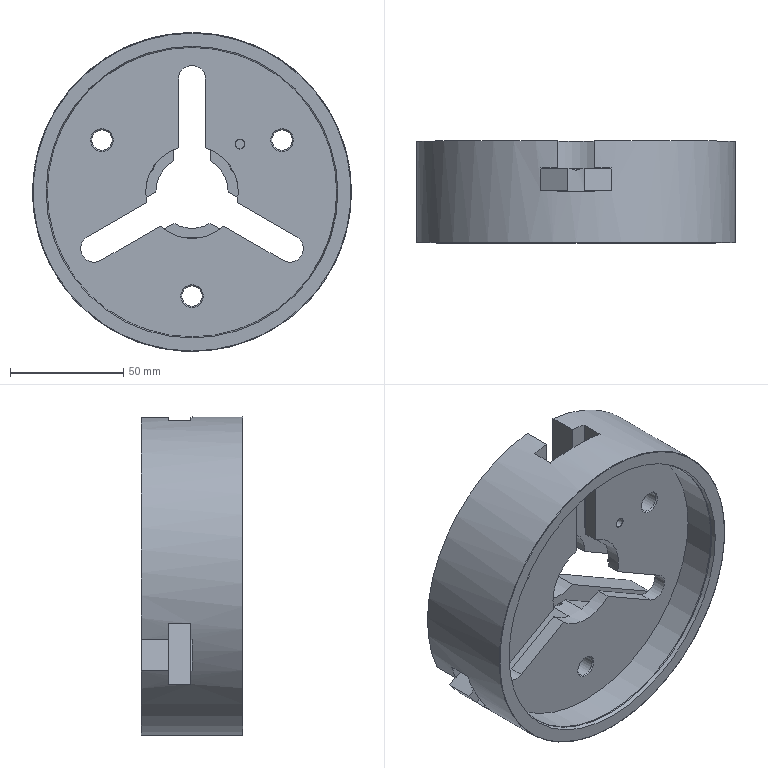NC program | NX | posted with a generic post | part box 141 x 45 x 141 mm
Whole program:
N10 G17 G21 G94 G90
(PLANAR_MILL_2_COPY , TOOL : D30)
N12 T07 M6
N14 G54
N16 G17 G0 G90 X0. Y110. S0 M3
N18 G43 Z100. H7
N20 Z-20.1
N22 G94 G1 Z-21.1 F250.
N24 Y80.
N26 X0.4
N28 Y15.1
N30 X-0.4
N32 Y80.
N34 X0.
N36 Y110.
N38 Z-20.1
N40 G0 Z-20.9
N42 G1 Z-21.9
N44 Y80.
N46 X0.4
N48 Y15.1
N50 X-0.4
N52 Y80.
N54 X0.
N56 Y110.
N58 Z-20.9
N60 G0 Z100.
(PLANAR_MILL_2_COPY_COPY , TOOL : D30)
N62 X-95.263 Y-55.
N64 Z-20.1
N66 G1 Z-21.1
N68 X-69.282 Y-40.
N70 X-69.482 Y-39.654
N72 X-13.277 Y-7.204
N74 X-12.877 Y-7.896
N76 X-69.082 Y-40.346
N78 X-69.282 Y-40.
N80 X-95.263 Y-55.
N82 Z-20.1
N84 G0 Z-20.9
N86 G1 Z-21.9
N88 X-69.282 Y-40.
N90 X-69.482 Y-39.654
N92 X-13.277 Y-7.204
N94 X-12.877 Y-7.896
N96 X-69.082 Y-40.346
N98 X-69.282 Y-40.
N100 X-95.263 Y-55.
N102 Z-20.9
N104 G0 Z100.
(PLANAR_MILL_2_COPY_COPY_1 , TOOL : D30)
N106 X95.263
N108 Z-20.1
N110 G1 Z-21.1
N112 X69.282 Y-40.
N114 X69.082 Y-40.346
N116 X12.877 Y-7.896
N118 X13.277 Y-7.204
N120 X69.482 Y-39.654
N122 X69.282 Y-40.
N124 X95.263 Y-55.
N126 Z-20.1
N128 G0 Z-20.9
N130 G1 Z-21.9
N132 X69.282 Y-40.
N134 X69.082 Y-40.346
N136 X12.877 Y-7.896
N138 X13.277 Y-7.204
N140 X69.482 Y-39.654
N142 X69.282 Y-40.
N144 X95.263 Y-55.
N146 Z-20.9
N148 G0 Z100.
N150 M5
N152 M2